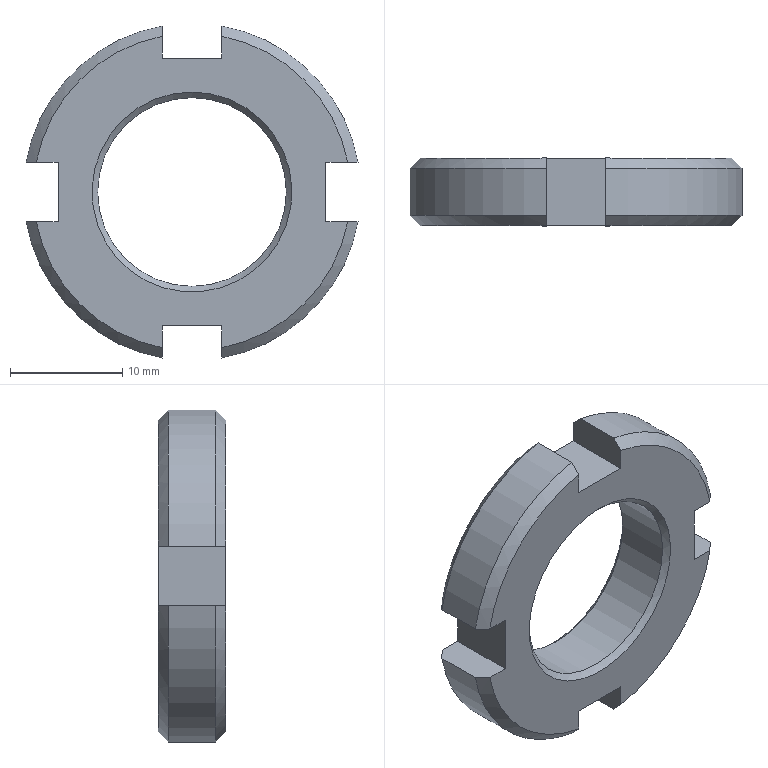Part | STEP file | Tube feed_id142_x_t | 1 solid | 29 faces | box 29.528 x 6 x 29.528 mm | volume 2459 mm3 | plane 14 | cone 10 | cylinder 5 | commonest cylinder face diameters 30 x4 16.782 x1